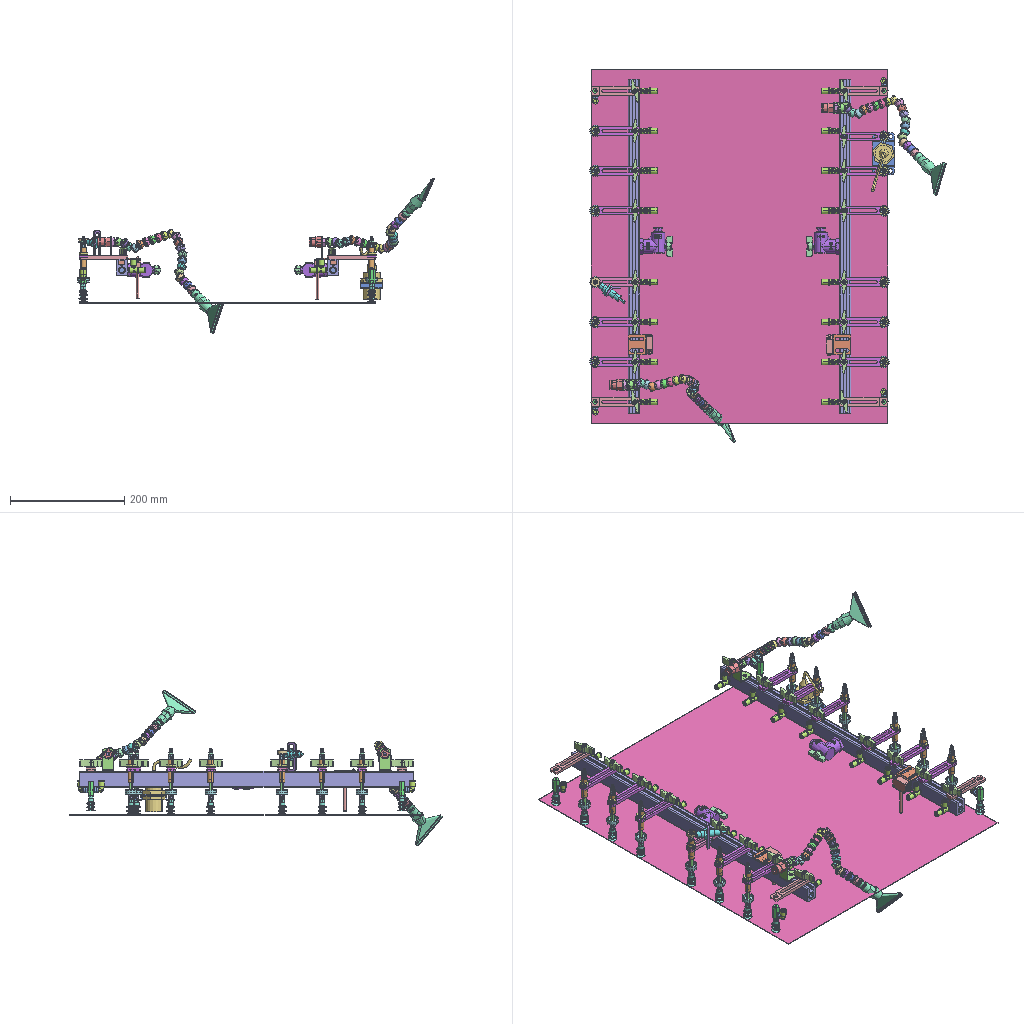Assembly | SolidWorks | 29 different items | 163 placed | box 625 x 653 x 273 mm
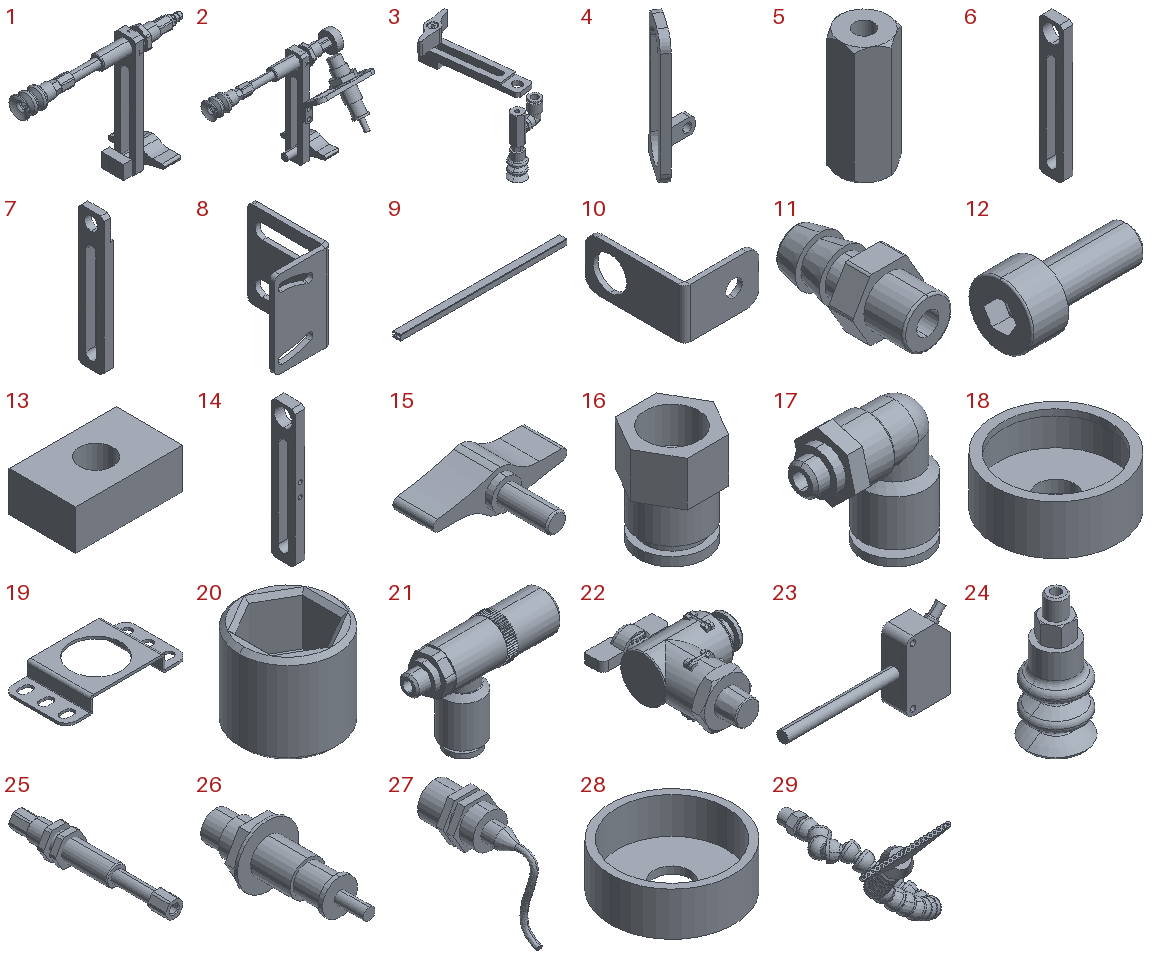Parts list (item | name | quantity | parent item | size | volume | features):
1 | (subassembly) | x11 | - | 115.5 x 39.995 x 85.247 mm | 15600 mm3 | -
2 | (subassembly) | x1 | - | 126 x 57.116 x 86 mm | 21560 mm3 | -
3 | (subassembly) | x4 | - | 50.199 x 85.818 x 89.5 mm | 14095 mm3 | -
4 | - | x1 | in 2 | 25.898 x 17.285 x 50 mm | 1263 mm3 | features Fillet 2, ICE 2, EdgeFlange 1, FlatPattern 1, HoleWzd 1, SMBaseFlange 1, SheetMetal 1
5 | - | x4 | in 3 | 10 x 11.547 x 25 mm | 1883 mm3 | features HoleWzd 3, RevCut 2, Extrusion 1, ICE 1
6 | - | x11 | in 1 | 6 x 15 x 85 mm | 4825 mm3 | features Chamfer 1, Extrusion 1, HoleWzd 1
7 | - | x4 | in 3 | 6 x 16 x 85 mm | 5085 mm3 | features Chamfer 1, Extrusion 1, HoleWzd 1, ICE 1
8 | - | x2 | - | 23 x 32 x 35 mm | 2932 mm3 | features ICE 2, Fillet 1, FlatPattern 1, HoleWzd 1, MirrorPattern 1, SMBaseFlange 1, SheetMetal 1
9 | - | x2 | - | 585 x 28 x 20 mm | 202510 mm3 | features HoleWzd 7, Extrusion 1, Fillet 1, ICE 1
10 | - | x2 | - | 30 x 40 x 20 mm | 2300 mm3 | features Fillet 1, FlatPattern 1, HoleWzd 1, ICE 1, SMBaseFlange 1, SheetMetal 1
11 | - | x12 | in 1, 2 | 7.24 x 13.6 x 6.35 mm | 219.147 mm3 | features ICE 5, Fillet 2, Extrusion 1
12 | - | x1 | - | 14 x 7 x 7 mm | 260.108 mm3 | features Fillet 2, RevCut 2, Attribute 1, Cut 1, LPattern 1, Revolution 1
13 | - | x15 | in 1, 3 | 16 x 10 x 6 mm | 842.19 mm3 | features Extrusion 1, HoleWzd 1
14 | - | x1 | in 2 | 6 x 15 x 85 mm | 4761 mm3 | features HoleWzd 2, Chamfer 1, Extrusion 1
15 | - | x16 | in 1, 2, 3 | 40 x 29 x 11.94 mm | 3436 mm3 | features ICE 10, Fillet 6, BaseBody 1, Chamfer 1, HoleWzd 1, MoveCopyBody 1, Stock 1
16 | - | x2 | - | 18.475 x 16 x 22 mm | 2877 mm3 | features ICE 4, Extrusion 1, HoleWzd 1
17 | - | x4 | in 3 | 20.75 x 10.5 x 21.285 mm | 1349 mm3 | features ICE 10, Chamfer 3, Extrusion 1, RevCut 1, Sweep 1
18 | - | x12 | - | 20 x 20 x 8 mm | 885.733 mm3 | features ICE 3, Extrusion 1
19 | - | x1 | - | 74 x 38 x 10 mm | 3632 mm3 | features EdgeFlange 2, Fillet 1, FlatPattern 1, HoleWzd 1, ICE 1, SMBaseFlange 1, SheetMetal 1
20 | - | x4 | - | 11.45 x 11.45 x 10.4 mm | 725.97 mm3 | features BaseBody 1
21 | - | x16 | - | 35 x 10.589 x 25.544 mm | 3217 mm3 | features ICE 13, Chamfer 4, CirPattern 1, Extrusion 1, Fillet 1, RevCut 1, Revolution 1, Sweep 1
22 | - | x2 | - | 50.7 x 68.7 x 25.6 mm | 31138 mm3 | features BaseBody 2
23 | - | x2 | - | 72.394 x 11.2 x 35.904 mm | 7657 mm3 | features Boss 4, Chamfer 3, Fillet 3, Cut 2, Dome 2, Extrusion 1, HoleWzd 1, ICE 1
24 | - | x16 | in 1, 2, 3 | 14.806 x 14.806 x 32 mm | 1500 mm3 | features BaseBody 1
25 | - | x12 | in 1, 2 | 15.5 x 79 x 14 mm | 4777 mm3 | features BaseBody 6
26 | - | x1 | in 2 | 21 x 52.5 x 21 mm | 5144 mm3 | features Boss 2, Revolution 1
27 | - | x1 | - | 40.415 x 92.567 x 87.046 mm | 43733 mm3 | features Boss 2, Extrusion 1, LPattern 1, Revolution 1, Sweep 1
28 | - | x1 | in 2 | 17 x 17 x 6 mm | 458.673 mm3 | features Extrusion 1, ICE 1
29 | - | x2 | - | 142.999 x 211.658 x 156.105 mm | 39289 mm3 | features BaseBody 25, Blend 2, ICE 2
Mates (type | each side: item.copy, entity, surface, feature):
In the top assembly
Coincident | 8.1 face plane Base-Flange1 | 23.1 face plane Extrude1
Concentric | 8.1 face cylinder M3 Clearance Hole1 | 23.1 face cylinder M3x0.5 Tapped Hole1
Coincident | 9.1 face plane Extrude1 | 8.1 face plane Base-Flange1
Coincident | 9.2 face plane Extrude1 | 9.1 face plane Extrude1 | 2 times
Concentric | 9.2 face cylinder G1/4 Tapped Hole2 | 20.1 face cylinder Input1
Coincident | 9.2 face plane Extrude1 | 20.1 face plane Input1
Concentric | 9.2 face cylinder G1/4 Tapped Hole1 | 20.2 face cylinder Input1
Coincident | 9.2 face plane Extrude1 | 20.2 face plane Input1
Concentric | 9.1 face cylinder G1/4 Tapped Hole1 | 20.3 face cylinder Input1
Coincident | 9.1 face plane Extrude1 | 20.3 face plane Input1
Concentric | 9.1 face cylinder G1/4 Tapped Hole2 | 20.4 face cylinder Input1
Coincident | 9.1 face plane Extrude1 | 20.4 face plane Input1
Concentric | 9.2 face cylinder M5 Tapped Hole2 | 21.1 face cylinder Boss-Extrude13
Coincident | 9.2 face plane Extrude1 | 21.1 face plane Boss-Extrude12
Coincident | 9.2 face plane Extrude1 | 21.2 face plane Boss-Extrude12
Concentric | 9.2 face cylinder M5 Tapped Hole2 | 21.2 face cylinder Boss-Extrude13
Coincident | 9.2 face plane Extrude1 | 21.3 face plane Boss-Extrude12
Concentric | 9.2 face cylinder M5 Tapped Hole2 | 21.3 face cylinder Boss-Extrude13
Coincident | 9.2 face plane Extrude1 | 21.4 face plane Boss-Extrude12
Concentric | 9.2 face cylinder M5 Tapped Hole2 | 21.4 face cylinder Boss-Extrude13
Coincident | 9.2 face plane Extrude1 | 21.5 face plane Boss-Extrude12
Concentric | 9.2 face cylinder M5 Tapped Hole2 | 21.5 face cylinder Boss-Extrude13
Coincident | 9.2 face plane Extrude1 | 21.6 face plane Boss-Extrude12
Concentric | 9.2 face cylinder M5 Tapped Hole2 | 21.6 face cylinder Boss-Extrude13
Coincident | 9.2 face plane Extrude1 | 21.7 face plane Boss-Extrude12
Concentric | 9.2 face cylinder M5 Tapped Hole2 | 21.7 face cylinder Boss-Extrude13
Coincident | 9.2 face plane Extrude1 | 21.8 face plane Boss-Extrude12
Concentric | 9.2 face cylinder M5 Tapped Hole2 | 21.8 face cylinder Boss-Extrude13
Parallel | 9.2 face plane Extrude1 | 21.1 face plane Boss-Extrude1
Parallel | 9.2 face plane Extrude1 | 21.2 face plane Boss-Extrude1
Parallel | 9.2 face plane Extrude1 | 21.3 face plane Boss-Extrude1
Parallel | 9.2 face plane Extrude1 | 21.4 face plane Boss-Extrude1
Parallel | 9.2 face plane Extrude1 | 21.8 face plane Boss-Extrude1
Parallel | 9.2 face plane Extrude1 | 21.7 face plane Boss-Extrude1
Parallel | 9.2 face plane Extrude1 | 21.6 face plane Boss-Extrude1
Parallel | 9.2 face plane Extrude1 | 21.5 face plane Boss-Extrude1
Concentric | 9.1 face cylinder M5 Tapped Hole2 | 21.9 face cylinder Boss-Extrude13
Coincident | 9.1 face plane Extrude1 | 21.9 face plane Boss-Extrude12
Parallel | 9.1 face plane Extrude1 | 21.9 face plane Boss-Extrude1
Coincident | 9.1 face plane Extrude1 | 21.10 face plane Boss-Extrude12
Parallel | 9.1 face plane Extrude1 | 21.10 face plane Boss-Extrude1
Concentric | 9.1 face cylinder M5 Tapped Hole2 | 21.10 face cylinder Boss-Extrude13
Coincident | 9.1 face plane Extrude1 | 21.11 face plane Boss-Extrude12
Parallel | 9.1 face plane Extrude1 | 21.11 face plane Boss-Extrude1
Concentric | 9.1 face cylinder M5 Tapped Hole2 | 21.11 face cylinder Boss-Extrude13
Coincident | 9.1 face plane Extrude1 | 21.12 face plane Boss-Extrude12
Parallel | 9.1 face plane Extrude1 | 21.12 face plane Boss-Extrude1
Concentric | 9.1 face cylinder M5 Tapped Hole2 | 21.12 face cylinder Boss-Extrude13
Coincident | 9.1 face plane Extrude1 | 21.13 face plane Boss-Extrude12
Parallel | 9.1 face plane Extrude1 | 21.13 face plane Boss-Extrude1
Concentric | 9.1 face cylinder M5 Tapped Hole2 | 21.13 face cylinder Boss-Extrude13
Coincident | 9.1 face plane Extrude1 | 21.14 face plane Boss-Extrude12
Parallel | 9.1 face plane Extrude1 | 21.14 face plane Boss-Extrude1
Concentric | 9.1 face cylinder M5 Tapped Hole2 | 21.14 face cylinder Boss-Extrude13
Coincident | 9.1 face plane Extrude1 | 21.15 face plane Boss-Extrude12
Parallel | 9.1 face plane Extrude1 | 21.15 face plane Boss-Extrude1
Concentric | 9.1 face cylinder M5 Tapped Hole2 | 21.15 face cylinder Boss-Extrude13
Coincident | 9.1 face plane Extrude1 | 21.16 face plane Boss-Extrude12
Parallel | 9.1 face plane Extrude1 | 21.16 face plane Boss-Extrude1
Concentric | 9.1 face cylinder M5 Tapped Hole2 | 21.16 face cylinder Boss-Extrude13
Coincident | 9.2 face plane Extrude1 | 7.1 face plane Extrude1 | 2 times
Parallel | 9.2 face plane Extrude1 | 7.1 face plane Extrude1
Coincident | 23.2 face plane Extrude1 | 8.2 face plane Base-Flange1 | 2 times
Parallel | 23.2 face plane Extrude1 | 8.2 face plane Base-Flange1
Coincident | 9.2 face plane Extrude1 | 6.1 face plane Extrude1 | 2 times
Width | 6.1 face plane Extrude1 | 6.1 face plane Extrude1 | 21.6 face cylinder Boss-Extrude10
Coincident | 9.2 face plane Extrude1 | 6.2 face plane Extrude1 | 2 times
Width | 6.2 face plane Extrude1 | 6.2 face plane Extrude1 | 21.7 face cylinder Boss-Extrude10
Coincident | 9.2 face plane Extrude1 | 6.3 face plane Extrude1 | 2 times
Width | 6.3 face plane Extrude1 | 6.3 face plane Extrude1 | 21.8 face cylinder Boss-Extrude10
Coincident | 9.2 face plane Extrude1 | 6.4 face plane Extrude1 | 2 times
Width | 6.4 face plane Extrude1 | 6.4 face plane Extrude1 | 21.4 face cylinder Boss-Extrude10
Coincident | 9.2 face plane Extrude1 | 6.5 face plane Extrude1 | 2 times
Width | 6.5 face plane Extrude1 | 6.5 face plane Extrude1 | 21.3 face cylinder Boss-Extrude10
Coincident | 9.2 face plane Extrude1 | 6.6 face plane Extrude1 | 2 times
Coincident | 9.1 face plane Extrude1 | 6.7 face plane Extrude1 | 2 times
Width | 6.7 face plane Extrude1 | 6.7 face plane Extrude1 | 21.15 face cylinder Boss-Extrude10
Coincident | 9.1 face plane Extrude1 | 6.8 face plane Extrude1 | 2 times
Width | 6.8 face plane Extrude1 | 6.8 face plane Extrude1 | 21.14 face cylinder Boss-Extrude10
Coincident | 9.1 face plane Extrude1 | 14.1 face plane Extrude1 | 2 times
Width | 14.1 face plane Extrude1 | 14.1 face plane Extrude1 | 21.13 face cylinder Boss-Extrude10
Coincident | 9.1 face plane Extrude1 | 6.9 face plane Extrude1 | 2 times
Width | 6.9 face plane Extrude1 | 6.9 face plane Extrude1 | 21.10 face cylinder Boss-Extrude10
Coincident | 9.1 face plane Extrude1 | 6.10 face plane Extrude1 | 2 times
Width | 6.10 face plane Extrude1 | 6.10 face plane Extrude1 | 21.12 face cylinder Boss-Extrude10
Coincident | 9.1 face plane Extrude1 | 6.11 face plane Extrude1 | 2 times
Width | 6.11 face plane Extrude1 | 6.11 face plane Extrude1 | 21.11 face cylinder Boss-Extrude10
Width | 7.1 face plane Extrude1 | 7.1 face plane Extrude1 | 21.1 face cylinder Boss-Extrude10
Coincident | 9.1 face plane Extrude1 | 7.2 face plane Extrude1 | 2 times
Width | 7.2 face plane Extrude1 | 7.2 face plane Extrude1 | 21.9 face cylinder Boss-Extrude10
Coincident | 9.1 face plane Extrude1 | 7.3 face plane Extrude1 | 2 times
Width | 7.3 face plane Extrude1 | 7.3 face plane Extrude1 | 21.16 face cylinder Boss-Extrude10
Coincident | 9.2 face plane Extrude1 | 7.4 face plane Extrude1 | 2 times
Width | 7.4 face plane Extrude1 | 7.4 face plane Extrude1 | 21.5 face cylinder Boss-Extrude10
Coincident | 9.2 face plane Extrude1 | 8.1 face plane Base-Flange1
Slot | 23.2 face cylinder M3x0.5 Tapped Hole1 | 8.2 face cylinder Mirror1
Coincident | 8.2 face plane Base-Flange1 | 9.1 face plane Extrude1 | 2 times
DistanceDim | 8.1 face plane Base-Flange1 | 6.1 face plane Extrude1
Coincident | 8.1 face plane Base-Flange1 | 8.2 face plane Base-Flange1
Coincident | 9.2 face plane Extrude1 | 10.1 face plane Base-Flange1 | 2 times
DistanceDim | 10.1 face plane Base-Flange1 | 9.2 face plane Extrude1
Coincident | 9.1 face plane Extrude1 | 10.2 face plane Base-Flange1 | 2 times
DistanceDim | 10.2 face plane Base-Flange1 | 9.1 face plane Extrude1
Concentric | 25.1 face cylinder Input3 | 18.1 face cylinder Boss-Extrude1
Coincident | 25.1 face plane Input2 | 18.1 face plane Boss-Extrude1
Concentric | 25.2 face cylinder Input3 | 18.2 face cylinder Boss-Extrude1
Coincident | 25.2 face plane Input2 | 18.2 face plane Boss-Extrude1
Concentric | 25.3 face cylinder Input3 | 18.3 face cylinder Boss-Extrude1
Coincident | 25.3 face plane Input2 | 18.3 face plane Boss-Extrude1
Concentric | 25.4 face cylinder Input3 | 18.4 face cylinder Boss-Extrude1
Coincident | 25.4 face plane Input2 | 18.4 face plane Boss-Extrude1
Concentric | 25.5 face cylinder Input3 | 18.5 face cylinder Boss-Extrude1
Coincident | 25.5 face plane Input2 | 18.5 face plane Boss-Extrude1
Concentric | 25.6 face cylinder Input3 | 18.6 face cylinder Boss-Extrude1
Coincident | 25.6 face plane Input2 | 18.6 face plane Boss-Extrude1
Concentric | 25.7 face cylinder Input3 | 18.7 face cylinder Boss-Extrude1
Coincident | 25.7 face plane Input2 | 18.7 face plane Boss-Extrude1
Concentric | 25.8 face cylinder Input3 | 18.8 face cylinder Boss-Extrude1
Coincident | 25.8 face plane Input2 | 18.8 face plane Boss-Extrude1
Concentric | 25.9 face cylinder Input3 | 18.9 face cylinder Boss-Extrude1
Coincident | 25.9 face plane Input2 | 18.9 face plane Boss-Extrude1
Concentric | 25.10 face cylinder Input3 | 18.10 face cylinder Boss-Extrude1
Coincident | 25.10 face plane Input2 | 18.10 face plane Boss-Extrude1
Concentric | 25.11 face cylinder Input3 | 18.11 face cylinder Boss-Extrude1
Coincident | 25.11 face plane Input2 | 18.11 face plane Boss-Extrude1
Concentric | 25.12 face cylinder Input3 | 18.12 face cylinder Boss-Extrude1
Coincident | 25.12 face plane Input2 | 18.12 face plane Boss-Extrude1
Concentric | 9.1 face cylinder G1/4 Tapped Hole7 | 22.1 face cone BVCEB10-2part1-1-solid1
Coincident | 9.1 face plane Extrude1 | 22.1 face plane BVCEB10-2part1-1-solid1
Parallel | 9.1 face plane Extrude1 | 22.1 face plane BVCEB10-2part1-1-solid1
Concentric | 9.2 face cylinder G1/4 Tapped Hole7 | 22.2 face cone BVCEB10-2part1-1-solid1
Coincident | 9.2 face plane Extrude1 | 22.2 face plane BVCEB10-2part1-1-solid1
Parallel | 9.2 face plane Extrude1 | 22.2 face plane BVCEB10-2part1-1-solid1
Concentric | 29.1 face cylinder Tail connector-1-solid1 | 16.1 face cylinder Boss-Extrude3
Coincident | 29.1 face plane Tail connector-1-solid1 | 16.1 face plane Boss-Extrude4
Concentric | 10.2 face cylinder Cut-Extrude1 | 16.1 face cylinder Boss-Extrude3
Concentric | 29.2 face cylinder Tail connector-1-solid1 | 16.2 face cylinder Boss-Extrude3
Coincident | 29.2 face plane Tail connector-1-solid1 | 16.2 face plane Boss-Extrude4
Concentric | 10.1 face cylinder Cut-Extrude1 | 16.2 face cylinder Boss-Extrude3
Coincident | 10.2 face plane Base-Flange1 | 16.1 face plane Boss-Extrude4
Coincident | 10.1 face plane Base-Flange1 | 16.2 face plane Boss-Extrude4
Coincident | 25.11 face plane Input2 | 19.1 face plane Edge-Flange2
Slot | 19.1 face cylinder M5 Clearance slot1 | 25.11 face cylinder Input3
Slot | 19.1 face cylinder M5 Clearance slot1 | 25.12 face cylinder Input3
Concentric | 27.1 face cylinder Revolve1 | 19.1 face cylinder Cut-Extrude1
Coincident | 27.1 face plane Extrude2 | 19.1 face plane Base-Flange1
In subassembly 1
Concentric | 25.13 face cylinder Input5 | 11.1 face cylinder Boss-Extrude5
Coincident | 25.13 face plane Input5 | 11.1 face plane Boss-Extrude1
Concentric | 6.12 face cylinder M12x1.0 Tapped Hole1 | 25.13 face cylinder Input1
DistanceDim | 25.13 face plane Input1 | 6.12 face plane Extrude1
Concentric | 25.13 face cylinder Input2 | 24.1 face cylinder Input1
Coincident | 25.13 face plane Input2 | 24.1 face plane Input1
Concentric | 6.12 face cylinder Extrude1 | 15.1 face cylinder Input1
Coincident | 6.12 face plane Extrude1 | 15.1 face plane Cut-Extrude2
Concentric | 15.1 face cylinder Input1 | 13.1 face cylinder M6 Tapped Hole1
Coincident | 15.1 face plane Cut-Extrude3 | 13.1 face plane Boss-Extrude1
Parallel | 6.12 face plane Extrude1 | 13.1 face plane Boss-Extrude1
In subassembly 3
Concentric | 3.1 face | 7.5 face cylinder Ø8.2 (8.2) Diameter Hole1
Coincident | 3.1 face | 7.5 face plane Cut-Extrude1
Parallel | 3.1 face | 7.5 face plane Cut-Extrude1
Concentric | 3.1 face | 5.1 face cylinder M4 Tapped Hole1
Coincident | 3.1 face | 5.1 face plane Boss-Extrude1
Concentric | 3.1 face | 24.1 face cone Input1
Concentric | 5.1 face cylinder M5 Tapped Hole2 | 17.1 face cylinder Boss-Extrude13
Coincident | 5.1 face plane Boss-Extrude1 | 17.1 face plane Boss-Extrude12
Parallel | 5.1 face plane Boss-Extrude1 | 17.1 face plane Boss-Extrude1
Parallel | 7.5 face plane Extrude1 | 5.1 face plane Boss-Extrude1
Coincident | 24.1 face plane Input1 | 5.1 face plane Boss-Extrude1
Concentric | 7.5 face cylinder Extrude1 | 15.1 face cylinder Input1
Coincident | 7.5 face plane Extrude1 | 15.1 face plane Cut-Extrude2
Concentric | 15.1 face cylinder Input1 | 13.1 face cylinder M6 Tapped Hole1
Coincident | 15.1 face plane Cut-Extrude3 | 13.1 face plane Boss-Extrude1
Parallel | 7.5 face plane Extrude1 | 13.1 face plane Boss-Extrude1
In subassembly 2
Concentric | 25.13 face cylinder Input5 | 11.1 face cylinder Boss-Extrude5
Coincident | 25.13 face plane Input5 | 11.1 face plane Boss-Extrude1
Concentric | 14.2 face cylinder M12x1.0 Tapped Hole1 | 25.13 face cylinder Input1
DistanceDim | 25.13 face plane Input1 | 14.2 face plane Extrude1
Concentric | 25.13 face cylinder Input2 | 24.1 face cylinder Input1
Coincident | 25.13 face plane Input2 | 24.1 face plane Input1
Concentric | 14.2 face cylinder Extrude1 | 15.1 face cylinder Input1
Coincident | 14.2 face plane Extrude1 | 15.1 face plane Cut-Extrude2
Coincident | 14.2 face plane Extrude1 | 4.1 face plane Base-Flange1
Concentric | 14.2 face cylinder M3 Tapped Hole1 | 4.1 face cylinder M3 Clearance Hole1 | 2 times
Slot | 26.1 face cylinder Revolve1 | 4.1 face plane Cut-Extrude1
Coincident | 4.1 face plane Edge-Flange1 | 26.1 face plane Extrude2
Concentric | 11.1 face cylinder Boss-Extrude2 | 28.1 face cylinder Boss-Extrude1
Parallel | 25.13 face plane Input5 | 28.1 face plane Boss-Extrude1
Coincident | 25.13 face plane Input5 | 28.1 face plane Boss-Extrude1